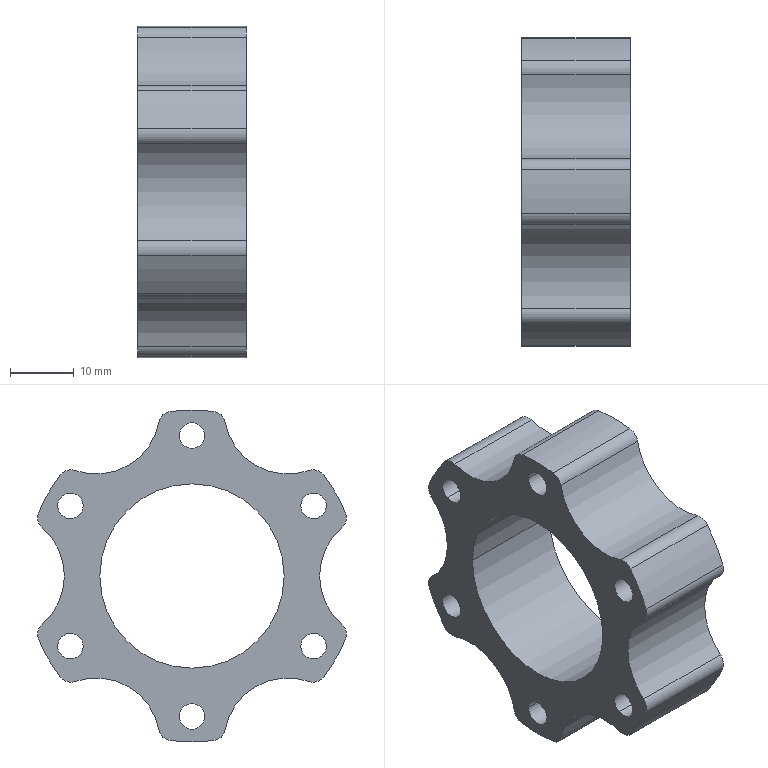Part | STEP file | BREP_88 | 1 solid | 40 faces | box 17 x 48.379 x 52 mm | volume 16406 mm3 | cylinder 38 | plane 2 | commonest cylinder face diameters 4 x24 20.148 x6 52 x6 28.87 x2